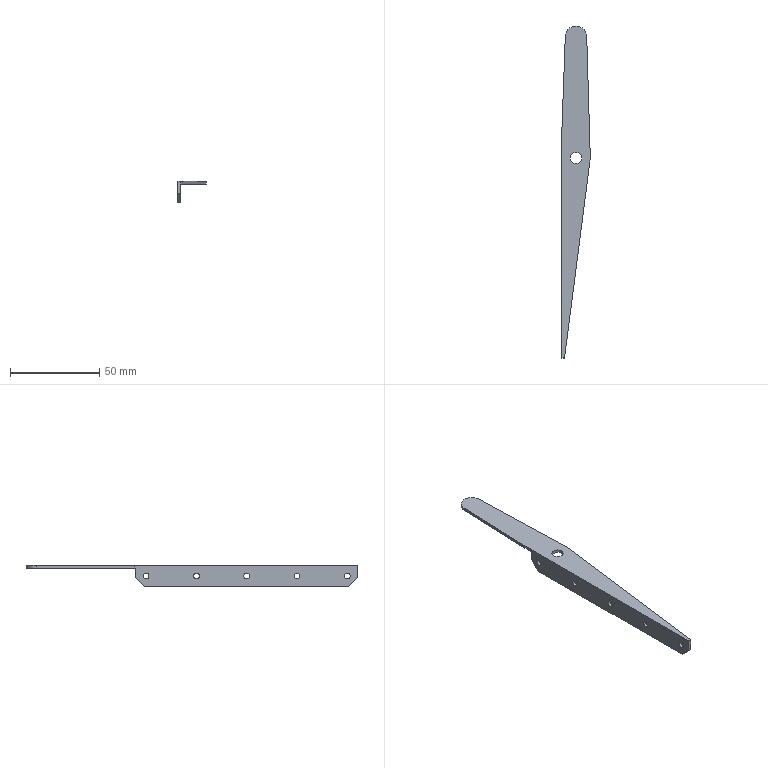Part | SolidWorks | features BaseBody 1 | 1 solid | 25 faces | box 16 x 185.958 x 12 mm | volume 5128 mm3 | cylinder 13 | plane 12 | commonest cylinder face diameters 3.2 x10 6.35 x2 12 x1
STEP:
#1=CARTESIAN_POINT('',(0.,90.45,-7.6));
#2=VERTEX_POINT('',#1);
#3=CARTESIAN_POINT('',(0.,90.45,-4.4));
#4=VERTEX_POINT('',#3);
#5=CARTESIAN_POINT('',(0.,90.45,-6.));
#6=DIRECTION('',(-1.,0.,0.));
#7=DIRECTION('',(0.,0.,-1.));
#8=AXIS2_PLACEMENT_3D('',#5,#6,#7);
#9=CIRCLE('',#8,1.6);
#10=EDGE_CURVE('',#2,#4,#9,.T.);
#11=ORIENTED_EDGE('',*,*,#10,.T.);
#12=CARTESIAN_POINT('',(1.6,90.45,-4.4));
#13=VERTEX_POINT('',#12);
#14=CARTESIAN_POINT('',(0.,90.45,-4.4));
#15=DIRECTION('',(1.,0.,0.));
#16=VECTOR('',#15,1000.);
#17=LINE('',#14,#16);
#18=EDGE_CURVE('',#4,#13,#17,.T.);
#19=ORIENTED_EDGE('',*,*,#18,.T.);
#20=CARTESIAN_POINT('',(1.6,90.45,-7.6));
#21=VERTEX_POINT('',#20);
#22=CARTESIAN_POINT('',(1.6,90.45,-6.));
#23=DIRECTION('',(1.,0.,0.));
#24=DIRECTION('',(0.,0.,-1.));
#25=AXIS2_PLACEMENT_3D('',#22,#23,#24);
#26=CIRCLE('',#25,1.6);
#27=EDGE_CURVE('',#13,#21,#26,.T.);
#28=ORIENTED_EDGE('',*,*,#27,.T.);
#29=CARTESIAN_POINT('',(0.,90.45,-7.6));
#30=DIRECTION('',(1.,0.,0.));
#31=VECTOR('',#30,1000.);
#32=LINE('',#29,#31);
#33=EDGE_CURVE('',#2,#21,#32,.T.);
#34=ORIENTED_EDGE('',*,*,#33,.F.);
#35=EDGE_LOOP('',(#11,#19,#28,#34));
#36=FACE_OUTER_BOUND('',#35,.T.);
#37=CARTESIAN_POINT('',(0.,90.45,-6.));
#38=DIRECTION('',(1.,0.,0.));
#39=DIRECTION('',(0.,0.,-1.));
#40=AXIS2_PLACEMENT_3D('',#37,#38,#39);
#41=CYLINDRICAL_SURFACE('',#40,1.6);
#42=ADVANCED_FACE('',(#36),#41,.F.);
#43=CARTESIAN_POINT('',(0.,118.645,-7.6));
#44=VERTEX_POINT('',#43);
#45=CARTESIAN_POINT('',(0.,118.645,-4.4));
#46=VERTEX_POINT('',#45);
#47=CARTESIAN_POINT('',(0.,118.645,-6.));
#48=DIRECTION('',(-1.,0.,0.));
#49=DIRECTION('',(0.,0.,-1.));
#50=AXIS2_PLACEMENT_3D('',#47,#48,#49);
#51=CIRCLE('',#50,1.6);
#52=EDGE_CURVE('',#44,#46,#51,.T.);
#53=ORIENTED_EDGE('',*,*,#52,.T.);
#54=CARTESIAN_POINT('',(1.6,118.645,-4.4));
#55=VERTEX_POINT('',#54);
#56=CARTESIAN_POINT('',(0.,118.645,-4.4));
#57=DIRECTION('',(1.,0.,0.));
#58=VECTOR('',#57,1000.);
#59=LINE('',#56,#58);
#60=EDGE_CURVE('',#46,#55,#59,.T.);
#61=ORIENTED_EDGE('',*,*,#60,.T.);
#62=CARTESIAN_POINT('',(1.6,118.645,-7.6));
#63=VERTEX_POINT('',#62);
#64=CARTESIAN_POINT('',(1.6,118.645,-6.));
#65=DIRECTION('',(1.,0.,0.));
#66=DIRECTION('',(0.,0.,-1.));
#67=AXIS2_PLACEMENT_3D('',#64,#65,#66);
#68=CIRCLE('',#67,1.6);
#69=EDGE_CURVE('',#55,#63,#68,.T.);
#70=ORIENTED_EDGE('',*,*,#69,.T.);
#71=CARTESIAN_POINT('',(0.,118.645,-7.6));
#72=DIRECTION('',(1.,0.,0.));
#73=VECTOR('',#72,1000.);
#74=LINE('',#71,#73);
#75=EDGE_CURVE('',#44,#63,#74,.T.);
#76=ORIENTED_EDGE('',*,*,#75,.F.);
#77=EDGE_LOOP('',(#53,#61,#70,#76));
#78=FACE_OUTER_BOUND('',#77,.T.);
#79=CARTESIAN_POINT('',(0.,118.645,-6.));
#80=DIRECTION('',(1.,0.,0.));
#81=DIRECTION('',(0.,0.,-1.));
#82=AXIS2_PLACEMENT_3D('',#79,#80,#81);
#83=CYLINDRICAL_SURFACE('',#82,1.6);
#84=ADVANCED_FACE('',(#78),#83,.F.);
#85=CARTESIAN_POINT('',(0.,34.15,-7.6));
#86=VERTEX_POINT('',#85);
#87=CARTESIAN_POINT('',(0.,34.15,-4.4));
#88=VERTEX_POINT('',#87);
#89=CARTESIAN_POINT('',(0.,34.15,-6.));
#90=DIRECTION('',(-1.,0.,0.));
#91=DIRECTION('',(0.,0.,-1.));
#92=AXIS2_PLACEMENT_3D('',#89,#90,#91);
#93=CIRCLE('',#92,1.6);
#94=EDGE_CURVE('',#86,#88,#93,.T.);
#95=ORIENTED_EDGE('',*,*,#94,.T.);
#96=CARTESIAN_POINT('',(1.6,34.15,-4.4));
#97=VERTEX_POINT('',#96);
#98=CARTESIAN_POINT('',(0.,34.15,-4.4));
#99=DIRECTION('',(1.,0.,0.));
#100=VECTOR('',#99,1000.);
#101=LINE('',#98,#100);
#102=EDGE_CURVE('',#88,#97,#101,.T.);
#103=ORIENTED_EDGE('',*,*,#102,.T.);
#104=CARTESIAN_POINT('',(1.6,34.15,-7.6));
#105=VERTEX_POINT('',#104);
#106=CARTESIAN_POINT('',(1.6,34.15,-6.));
#107=DIRECTION('',(1.,0.,0.));
#108=DIRECTION('',(0.,0.,-1.));
#109=AXIS2_PLACEMENT_3D('',#106,#107,#108);
#110=CIRCLE('',#109,1.6);
#111=EDGE_CURVE('',#97,#105,#110,.T.);
#112=ORIENTED_EDGE('',*,*,#111,.T.);
#113=CARTESIAN_POINT('',(0.,34.15,-7.6));
#114=DIRECTION('',(1.,0.,0.));
#115=VECTOR('',#114,1000.);
#116=LINE('',#113,#115);
#117=EDGE_CURVE('',#86,#105,#116,.T.);
#118=ORIENTED_EDGE('',*,*,#117,.F.);
#119=EDGE_LOOP('',(#95,#103,#112,#118));
#120=FACE_OUTER_BOUND('',#119,.T.);
#121=CARTESIAN_POINT('',(0.,34.15,-6.));
#122=DIRECTION('',(1.,0.,0.));
#123=DIRECTION('',(0.,0.,-1.));
#124=AXIS2_PLACEMENT_3D('',#121,#122,#123);
#125=CYLINDRICAL_SURFACE('',#124,1.6);
#126=ADVANCED_FACE('',(#120),#125,.F.);
#127=CARTESIAN_POINT('',(0.,6.,-7.6));
#128=VERTEX_POINT('',#127);
#129=CARTESIAN_POINT('',(0.,6.,-4.4));
#130=VERTEX_POINT('',#129);
#131=CARTESIAN_POINT('',(0.,6.,-6.));
#132=DIRECTION('',(-1.,0.,0.));
#133=DIRECTION('',(0.,0.,-1.));
#134=AXIS2_PLACEMENT_3D('',#131,#132,#133);
#135=CIRCLE('',#134,1.6);
#136=EDGE_CURVE('',#128,#130,#135,.T.);
#137=ORIENTED_EDGE('',*,*,#136,.T.);
#138=CARTESIAN_POINT('',(1.6,6.,-4.4));
#139=VERTEX_POINT('',#138);
#140=CARTESIAN_POINT('',(0.,6.,-4.4));
#141=DIRECTION('',(1.,0.,0.));
#142=VECTOR('',#141,1000.);
#143=LINE('',#140,#142);
#144=EDGE_CURVE('',#130,#139,#143,.T.);
#145=ORIENTED_EDGE('',*,*,#144,.T.);
#146=CARTESIAN_POINT('',(1.6,6.,-7.6));
#147=VERTEX_POINT('',#146);
#148=CARTESIAN_POINT('',(1.6,6.,-6.));
#149=DIRECTION('',(1.,0.,0.));
#150=DIRECTION('',(0.,0.,-1.));
#151=AXIS2_PLACEMENT_3D('',#148,#149,#150);
#152=CIRCLE('',#151,1.6);
#153=EDGE_CURVE('',#139,#147,#152,.T.);
#154=ORIENTED_EDGE('',*,*,#153,.T.);
#155=CARTESIAN_POINT('',(0.,6.,-7.6));
#156=DIRECTION('',(1.,0.,0.));
#157=VECTOR('',#156,1000.);
#158=LINE('',#155,#157);
#159=EDGE_CURVE('',#128,#147,#158,.T.);
#160=ORIENTED_EDGE('',*,*,#159,.F.);
#161=EDGE_LOOP('',(#137,#145,#154,#160));
#162=FACE_OUTER_BOUND('',#161,.T.);
#163=CARTESIAN_POINT('',(0.,6.,-6.));
#164=DIRECTION('',(1.,0.,0.));
#165=DIRECTION('',(0.,0.,-1.));
#166=AXIS2_PLACEMENT_3D('',#163,#164,#165);
#167=CYLINDRICAL_SURFACE('',#166,1.6);
#168=ADVANCED_FACE('',(#162),#167,.F.);
#169=CARTESIAN_POINT('',(0.,62.3,-7.6));
#170=VERTEX_POINT('',#169);
#171=CARTESIAN_POINT('',(0.,62.3,-4.4));
#172=VERTEX_POINT('',#171);
#173=CARTESIAN_POINT('',(0.,62.3,-6.));
#174=DIRECTION('',(-1.,0.,0.));
#175=DIRECTION('',(0.,0.,-1.));
#176=AXIS2_PLACEMENT_3D('',#173,#174,#175);
#177=CIRCLE('',#176,1.6);
#178=EDGE_CURVE('',#170,#172,#177,.T.);
#179=ORIENTED_EDGE('',*,*,#178,.T.);
#180=CARTESIAN_POINT('',(1.6,62.3,-4.4));
#181=VERTEX_POINT('',#180);
#182=CARTESIAN_POINT('',(0.,62.3,-4.4));
#183=DIRECTION('',(1.,0.,0.));
#184=VECTOR('',#183,1000.);
#185=LINE('',#182,#184);
#186=EDGE_CURVE('',#172,#181,#185,.T.);
#187=ORIENTED_EDGE('',*,*,#186,.T.);
#188=CARTESIAN_POINT('',(1.6,62.3,-7.6));
#189=VERTEX_POINT('',#188);
#190=CARTESIAN_POINT('',(1.6,62.3,-6.));
#191=DIRECTION('',(1.,0.,0.));
#192=DIRECTION('',(0.,0.,-1.));
#193=AXIS2_PLACEMENT_3D('',#190,#191,#192);
#194=CIRCLE('',#193,1.6);
#195=EDGE_CURVE('',#181,#189,#194,.T.);
#196=ORIENTED_EDGE('',*,*,#195,.T.);
#197=CARTESIAN_POINT('',(0.,62.3,-7.6));
#198=DIRECTION('',(1.,0.,0.));
#199=VECTOR('',#198,1000.);
#200=LINE('',#197,#199);
#201=EDGE_CURVE('',#170,#189,#200,.T.);
#202=ORIENTED_EDGE('',*,*,#201,.F.);
#203=EDGE_LOOP('',(#179,#187,#196,#202));
#204=FACE_OUTER_BOUND('',#203,.T.);
#205=CARTESIAN_POINT('',(0.,62.3,-6.));
#206=DIRECTION('',(1.,0.,0.));
#207=DIRECTION('',(0.,0.,-1.));
#208=AXIS2_PLACEMENT_3D('',#205,#206,#207);
#209=CYLINDRICAL_SURFACE('',#208,1.6);
#210=ADVANCED_FACE('',(#204),#209,.F.);
#211=CARTESIAN_POINT('',(4.825,112.,0.));
#212=VERTEX_POINT('',#211);
#213=CARTESIAN_POINT('',(11.175,112.,0.));
#214=VERTEX_POINT('',#213);
#215=CARTESIAN_POINT('',(8.,112.,0.));
#216=DIRECTION('',(0.,0.,1.));
#217=DIRECTION('',(-1.,0.,0.));
#218=AXIS2_PLACEMENT_3D('',#215,#216,#217);
#219=CIRCLE('',#218,3.175);
#220=EDGE_CURVE('',#212,#214,#219,.T.);
#221=ORIENTED_EDGE('',*,*,#220,.T.);
#222=CARTESIAN_POINT('',(11.175,112.,-1.6));
#223=VERTEX_POINT('',#222);
#224=CARTESIAN_POINT('',(11.175,112.,0.));
#225=DIRECTION('',(0.,0.,-1.));
#226=VECTOR('',#225,1000.);
#227=LINE('',#224,#226);
#228=EDGE_CURVE('',#214,#223,#227,.T.);
#229=ORIENTED_EDGE('',*,*,#228,.T.);
#230=CARTESIAN_POINT('',(4.825,112.,-1.6));
#231=VERTEX_POINT('',#230);
#232=CARTESIAN_POINT('',(8.,112.,-1.6));
#233=DIRECTION('',(0.,0.,-1.));
#234=DIRECTION('',(-1.,0.,0.));
#235=AXIS2_PLACEMENT_3D('',#232,#233,#234);
#236=CIRCLE('',#235,3.175);
#237=EDGE_CURVE('',#223,#231,#236,.T.);
#238=ORIENTED_EDGE('',*,*,#237,.T.);
#239=CARTESIAN_POINT('',(4.825,112.,0.));
#240=DIRECTION('',(0.,0.,-1.));
#241=VECTOR('',#240,1000.);
#242=LINE('',#239,#241);
#243=EDGE_CURVE('',#212,#231,#242,.T.);
#244=ORIENTED_EDGE('',*,*,#243,.F.);
#245=EDGE_LOOP('',(#221,#229,#238,#244));
#246=FACE_OUTER_BOUND('',#245,.T.);
#247=CARTESIAN_POINT('',(8.,112.,0.));
#248=DIRECTION('',(0.,0.,-1.));
#249=DIRECTION('',(-1.,0.,0.));
#250=AXIS2_PLACEMENT_3D('',#247,#248,#249);
#251=CYLINDRICAL_SURFACE('',#250,3.175);
#252=ADVANCED_FACE('',(#246),#251,.F.);
#253=ORIENTED_EDGE('',*,*,#18,.F.);
#254=CARTESIAN_POINT('',(0.,90.45,-6.));
#255=DIRECTION('',(-1.,0.,0.));
#256=DIRECTION('',(0.,0.,-1.));
#257=AXIS2_PLACEMENT_3D('',#254,#255,#256);
#258=CIRCLE('',#257,1.6);
#259=EDGE_CURVE('',#4,#2,#258,.T.);
#260=ORIENTED_EDGE('',*,*,#259,.T.);
#261=ORIENTED_EDGE('',*,*,#33,.T.);
#262=CARTESIAN_POINT('',(1.6,90.45,-6.));
#263=DIRECTION('',(1.,0.,0.));
#264=DIRECTION('',(0.,0.,-1.));
#265=AXIS2_PLACEMENT_3D('',#262,#263,#264);
#266=CIRCLE('',#265,1.6);
#267=EDGE_CURVE('',#21,#13,#266,.T.);
#268=ORIENTED_EDGE('',*,*,#267,.T.);
#269=EDGE_LOOP('',(#253,#260,#261,#268));
#270=FACE_OUTER_BOUND('',#269,.T.);
#271=CARTESIAN_POINT('',(0.,90.45,-6.));
#272=DIRECTION('',(1.,0.,0.));
#273=DIRECTION('',(0.,0.,-1.));
#274=AXIS2_PLACEMENT_3D('',#271,#272,#273);
#275=CYLINDRICAL_SURFACE('',#274,1.6);
#276=ADVANCED_FACE('',(#270),#275,.F.);
#277=CARTESIAN_POINT('',(1.6,118.645,-6.));
#278=DIRECTION('',(1.,0.,0.));
#279=DIRECTION('',(0.,0.,-1.));
#280=AXIS2_PLACEMENT_3D('',#277,#278,#279);
#281=CIRCLE('',#280,1.6);
#282=EDGE_CURVE('',#63,#55,#281,.T.);
#283=ORIENTED_EDGE('',*,*,#282,.F.);
#284=ORIENTED_EDGE('',*,*,#69,.F.);
#285=EDGE_LOOP('',(#283,#284));
#286=FACE_BOUND('',#285,.T.);
#287=CARTESIAN_POINT('',(1.6,34.15,-6.));
#288=DIRECTION('',(1.,0.,0.));
#289=DIRECTION('',(0.,0.,-1.));
#290=AXIS2_PLACEMENT_3D('',#287,#288,#289);
#291=CIRCLE('',#290,1.6);
#292=EDGE_CURVE('',#105,#97,#291,.T.);
#293=ORIENTED_EDGE('',*,*,#292,.F.);
#294=ORIENTED_EDGE('',*,*,#111,.F.);
#295=EDGE_LOOP('',(#293,#294));
#296=FACE_BOUND('',#295,.T.);
#297=CARTESIAN_POINT('',(1.6,6.,-6.));
#298=DIRECTION('',(1.,0.,0.));
#299=DIRECTION('',(0.,0.,-1.));
#300=AXIS2_PLACEMENT_3D('',#297,#298,#299);
#301=CIRCLE('',#300,1.6);
#302=EDGE_CURVE('',#147,#139,#301,.T.);
#303=ORIENTED_EDGE('',*,*,#302,.F.);
#304=ORIENTED_EDGE('',*,*,#153,.F.);
#305=EDGE_LOOP('',(#303,#304));
#306=FACE_BOUND('',#305,.T.);
#307=CARTESIAN_POINT('',(1.6,62.3,-6.));
#308=DIRECTION('',(1.,0.,0.));
#309=DIRECTION('',(0.,0.,-1.));
#310=AXIS2_PLACEMENT_3D('',#307,#308,#309);
#311=CIRCLE('',#310,1.6);
#312=EDGE_CURVE('',#189,#181,#311,.T.);
#313=ORIENTED_EDGE('',*,*,#312,.F.);
#314=ORIENTED_EDGE('',*,*,#195,.F.);
#315=EDGE_LOOP('',(#313,#314));
#316=FACE_BOUND('',#315,.T.);
#317=ORIENTED_EDGE('',*,*,#267,.F.);
#318=ORIENTED_EDGE('',*,*,#27,.F.);
#319=EDGE_LOOP('',(#317,#318));
#320=FACE_BOUND('',#319,.T.);
#321=CARTESIAN_POINT('',(1.6,0.,-6.8));
#322=VERTEX_POINT('',#321);
#323=CARTESIAN_POINT('',(1.6,0.,-1.6));
#324=VERTEX_POINT('',#323);
#325=CARTESIAN_POINT('',(1.6,0.,-6.8));
#326=DIRECTION('',(0.,0.,1.));
#327=VECTOR('',#326,1000.);
#328=LINE('',#325,#327);
#329=EDGE_CURVE('',#322,#324,#328,.T.);
#330=ORIENTED_EDGE('',*,*,#329,.F.);
#331=CARTESIAN_POINT('',(1.6,5.2,-12.));
#332=VERTEX_POINT('',#331);
#333=CARTESIAN_POINT('',(1.6,0.,-6.8));
#334=DIRECTION('',(0.,-0.7071,0.7071));
#335=VECTOR('',#334,1000.);
#336=LINE('',#333,#335);
#337=EDGE_CURVE('',#332,#322,#336,.T.);
#338=ORIENTED_EDGE('',*,*,#337,.F.);
#339=CARTESIAN_POINT('',(1.6,119.8,-12.));
#340=VERTEX_POINT('',#339);
#341=CARTESIAN_POINT('',(1.6,62.323,-12.));
#342=DIRECTION('',(0.,-1.,0.));
#343=VECTOR('',#342,1000.);
#344=LINE('',#341,#343);
#345=EDGE_CURVE('',#340,#332,#344,.T.);
#346=ORIENTED_EDGE('',*,*,#345,.F.);
#347=CARTESIAN_POINT('',(1.6,124.645,-6.801));
#348=VERTEX_POINT('',#347);
#349=CARTESIAN_POINT('',(1.6,119.8,-12.));
#350=DIRECTION('',(0.,-0.6818,-0.7316));
#351=VECTOR('',#350,1000.);
#352=LINE('',#349,#351);
#353=EDGE_CURVE('',#348,#340,#352,.T.);
#354=ORIENTED_EDGE('',*,*,#353,.F.);
#355=CARTESIAN_POINT('',(1.6,124.645,-1.6));
#356=VERTEX_POINT('',#355);
#357=CARTESIAN_POINT('',(1.6,124.645,-6.8));
#358=DIRECTION('',(0.,0.,-1.));
#359=VECTOR('',#358,1000.);
#360=LINE('',#357,#359);
#361=EDGE_CURVE('',#356,#348,#360,.T.);
#362=ORIENTED_EDGE('',*,*,#361,.F.);
#363=CARTESIAN_POINT('',(1.6,62.323,-1.6));
#364=DIRECTION('',(0.,1.,0.));
#365=VECTOR('',#364,1000.);
#366=LINE('',#363,#365);
#367=EDGE_CURVE('',#324,#356,#366,.T.);
#368=ORIENTED_EDGE('',*,*,#367,.F.);
#369=EDGE_LOOP('',(#330,#338,#346,#354,#362,#368));
#370=FACE_OUTER_BOUND('',#369,.T.);
#371=CARTESIAN_POINT('',(1.6,124.645,-1.6));
#372=DIRECTION('',(-1.,0.,0.));
#373=DIRECTION('',(0.,0.,-1.));
#374=AXIS2_PLACEMENT_3D('',#371,#372,#373);
#375=PLANE('',#374);
#376=ADVANCED_FACE('',(#286,#296,#306,#316,#320,#370),#375,.F.);
#377=ORIENTED_EDGE('',*,*,#52,.F.);
#378=CARTESIAN_POINT('',(0.,118.645,-6.));
#379=DIRECTION('',(-1.,0.,0.));
#380=DIRECTION('',(0.,0.,-1.));
#381=AXIS2_PLACEMENT_3D('',#378,#379,#380);
#382=CIRCLE('',#381,1.6);
#383=EDGE_CURVE('',#46,#44,#382,.T.);
#384=ORIENTED_EDGE('',*,*,#383,.F.);
#385=EDGE_LOOP('',(#377,#384));
#386=FACE_BOUND('',#385,.T.);
#387=ORIENTED_EDGE('',*,*,#94,.F.);
#388=CARTESIAN_POINT('',(0.,34.15,-6.));
#389=DIRECTION('',(-1.,0.,0.));
#390=DIRECTION('',(0.,0.,-1.));
#391=AXIS2_PLACEMENT_3D('',#388,#389,#390);
#392=CIRCLE('',#391,1.6);
#393=EDGE_CURVE('',#88,#86,#392,.T.);
#394=ORIENTED_EDGE('',*,*,#393,.F.);
#395=EDGE_LOOP('',(#387,#394));
#396=FACE_BOUND('',#395,.T.);
#397=ORIENTED_EDGE('',*,*,#136,.F.);
#398=CARTESIAN_POINT('',(0.,6.,-6.));
#399=DIRECTION('',(-1.,0.,0.));
#400=DIRECTION('',(0.,0.,-1.));
#401=AXIS2_PLACEMENT_3D('',#398,#399,#400);
#402=CIRCLE('',#401,1.6);
#403=EDGE_CURVE('',#130,#128,#402,.T.);
#404=ORIENTED_EDGE('',*,*,#403,.F.);
#405=EDGE_LOOP('',(#397,#404));
#406=FACE_BOUND('',#405,.T.);
#407=ORIENTED_EDGE('',*,*,#178,.F.);
#408=CARTESIAN_POINT('',(0.,62.3,-6.));
#409=DIRECTION('',(-1.,0.,0.));
#410=DIRECTION('',(0.,0.,-1.));
#411=AXIS2_PLACEMENT_3D('',#408,#409,#410);
#412=CIRCLE('',#411,1.6);
#413=EDGE_CURVE('',#172,#170,#412,.T.);
#414=ORIENTED_EDGE('',*,*,#413,.F.);
#415=EDGE_LOOP('',(#407,#414));
#416=FACE_BOUND('',#415,.T.);
#417=ORIENTED_EDGE('',*,*,#10,.F.);
#418=ORIENTED_EDGE('',*,*,#259,.F.);
#419=EDGE_LOOP('',(#417,#418));
#420=FACE_BOUND('',#419,.T.);
#421=CARTESIAN_POINT('',(0.,119.8,-12.));
#422=VERTEX_POINT('',#421);
#423=CARTESIAN_POINT('',(0.,124.645,-6.801));
#424=VERTEX_POINT('',#423);
#425=CARTESIAN_POINT('',(0.,119.8,-12.));
#426=DIRECTION('',(0.,0.6818,0.7316));
#427=VECTOR('',#426,1000.);
#428=LINE('',#425,#427);
#429=EDGE_CURVE('',#422,#424,#428,.T.);
#430=ORIENTED_EDGE('',*,*,#429,.F.);
#431=CARTESIAN_POINT('',(0.,5.2,-12.));
#432=VERTEX_POINT('',#431);
#433=CARTESIAN_POINT('',(0.,62.5,-12.));
#434=DIRECTION('',(0.,1.,0.));
#435=VECTOR('',#434,1000.);
#436=LINE('',#433,#435);
#437=EDGE_CURVE('',#432,#422,#436,.T.);
#438=ORIENTED_EDGE('',*,*,#437,.F.);
#439=CARTESIAN_POINT('',(0.,0.,-6.8));
#440=VERTEX_POINT('',#439);
#441=CARTESIAN_POINT('',(0.,0.,-6.8));
#442=DIRECTION('',(0.,0.7071,-0.7071));
#443=VECTOR('',#442,1000.);
#444=LINE('',#441,#443);
#445=EDGE_CURVE('',#440,#432,#444,.T.);
#446=ORIENTED_EDGE('',*,*,#445,.F.);
#447=CARTESIAN_POINT('',(0.,0.,0.));
#448=VERTEX_POINT('',#447);
#449=CARTESIAN_POINT('',(0.,0.,-6.));
#450=DIRECTION('',(0.,0.,-1.));
#451=VECTOR('',#450,1000.);
#452=LINE('',#449,#451);
#453=EDGE_CURVE('',#448,#440,#452,.T.);
#454=ORIENTED_EDGE('',*,*,#453,.F.);
#455=CARTESIAN_POINT('',(0.,125.,0.));
#456=VERTEX_POINT('',#455);
#457=CARTESIAN_POINT('',(0.,62.5,0.));
#458=DIRECTION('',(0.,-1.,0.));
#459=VECTOR('',#458,1000.);
#460=LINE('',#457,#459);
#461=EDGE_CURVE('',#456,#448,#460,.T.);
#462=ORIENTED_EDGE('',*,*,#461,.F.);
#463=CARTESIAN_POINT('',(0.,125.,-1.6));
#464=VERTEX_POINT('',#463);
#465=CARTESIAN_POINT('',(0.,125.,-0.8));
#466=DIRECTION('',(0.,0.,-1.));
#467=VECTOR('',#466,1000.);
#468=LINE('',#465,#467);
#469=EDGE_CURVE('',#456,#464,#468,.T.);
#470=ORIENTED_EDGE('',*,*,#469,.T.);
#471=CARTESIAN_POINT('',(0.,124.645,-1.6));
#472=VERTEX_POINT('',#471);
#473=CARTESIAN_POINT('',(0.,62.5,-1.6));
#474=DIRECTION('',(0.,1.,0.));
#475=VECTOR('',#474,1000.);
#476=LINE('',#473,#475);
#477=EDGE_CURVE('',#472,#464,#476,.T.);
#478=ORIENTED_EDGE('',*,*,#477,.F.);
#479=CARTESIAN_POINT('',(0.,124.645,-6.));
#480=DIRECTION('',(0.,0.,1.));
#481=VECTOR('',#480,1000.);
#482=LINE('',#479,#481);
#483=EDGE_CURVE('',#424,#472,#482,.T.);
#484=ORIENTED_EDGE('',*,*,#483,.F.);
#485=EDGE_LOOP('',(#430,#438,#446,#454,#462,#470,#478,#484));
#486=FACE_OUTER_BOUND('',#485,.T.);
#487=CARTESIAN_POINT('',(0.,125.,-12.));
#488=DIRECTION('',(1.,0.,0.));
#489=DIRECTION('',(0.,0.,1.));
#490=AXIS2_PLACEMENT_3D('',#487,#488,#489);
#491=PLANE('',#490);
#492=ADVANCED_FACE('',(#386,#396,#406,#416,#420,#486),#491,.F.);
#493=ORIENTED_EDGE('',*,*,#60,.F.);
#494=ORIENTED_EDGE('',*,*,#383,.T.);
#495=ORIENTED_EDGE('',*,*,#75,.T.);
#496=ORIENTED_EDGE('',*,*,#282,.T.);
#497=EDGE_LOOP('',(#493,#494,#495,#496));
#498=FACE_OUTER_BOUND('',#497,.T.);
#499=CARTESIAN_POINT('',(0.,118.645,-6.));
#500=DIRECTION('',(1.,0.,0.));
#501=DIRECTION('',(0.,0.,-1.));
#502=AXIS2_PLACEMENT_3D('',#499,#500,#501);
#503=CYLINDRICAL_SURFACE('',#502,1.6);
#504=ADVANCED_FACE('',(#498),#503,.F.);
#505=ORIENTED_EDGE('',*,*,#102,.F.);
#506=ORIENTED_EDGE('',*,*,#393,.T.);
#507=ORIENTED_EDGE('',*,*,#117,.T.);
#508=ORIENTED_EDGE('',*,*,#292,.T.);
#509=EDGE_LOOP('',(#505,#506,#507,#508));
#510=FACE_OUTER_BOUND('',#509,.T.);
#511=CARTESIAN_POINT('',(0.,34.15,-6.));
#512=DIRECTION('',(1.,0.,0.));
#513=DIRECTION('',(0.,0.,-1.));
#514=AXIS2_PLACEMENT_3D('',#511,#512,#513);
#515=CYLINDRICAL_SURFACE('',#514,1.6);
#516=ADVANCED_FACE('',(#510),#515,.F.);
#517=ORIENTED_EDGE('',*,*,#144,.F.);
#518=ORIENTED_EDGE('',*,*,#403,.T.);
#519=ORIENTED_EDGE('',*,*,#159,.T.);
#520=ORIENTED_EDGE('',*,*,#302,.T.);
#521=EDGE_LOOP('',(#517,#518,#519,#520));
#522=FACE_OUTER_BOUND('',#521,.T.);
#523=CARTESIAN_POINT('',(0.,6.,-6.));
#524=DIRECTION('',(1.,0.,0.));
#525=DIRECTION('',(0.,0.,-1.));
#526=AXIS2_PLACEMENT_3D('',#523,#524,#525);
#527=CYLINDRICAL_SURFACE('',#526,1.6);
#528=ADVANCED_FACE('',(#522),#527,.F.);
#529=ORIENTED_EDGE('',*,*,#186,.F.);
#530=ORIENTED_EDGE('',*,*,#413,.T.);
#531=ORIENTED_EDGE('',*,*,#201,.T.);
#532=ORIENTED_EDGE('',*,*,#312,.T.);
#533=EDGE_LOOP('',(#529,#530,#531,#532));
#534=FACE_OUTER_BOUND('',#533,.T.);
#535=CARTESIAN_POINT('',(0.,62.3,-6.));
#536=DIRECTION('',(1.,0.,0.));
#537=DIRECTION('',(0.,0.,-1.));
#538=AXIS2_PLACEMENT_3D('',#535,#536,#537);
#539=CYLINDRICAL_SURFACE('',#538,1.6);
#540=ADVANCED_FACE('',(#534),#539,.F.);
#541=CARTESIAN_POINT('',(8.,112.,-1.6));
#542=DIRECTION('',(0.,0.,-1.));
#543=DIRECTION('',(-1.,0.,0.));
#544=AXIS2_PLACEMENT_3D('',#541,#542,#543);
#545=CIRCLE('',#544,3.175);
#546=EDGE_CURVE('',#231,#223,#545,.T.);
#547=ORIENTED_EDGE('',*,*,#546,.F.);
#548=ORIENTED_EDGE('',*,*,#237,.F.);
#549=EDGE_LOOP('',(#547,#548));
#550=FACE_BOUND('',#549,.T.);
#551=CARTESIAN_POINT('',(14.,179.958,-1.6));
#552=VERTEX_POINT('',#551);
#553=CARTESIAN_POINT('',(2.,179.958,-1.6));
#554=VERTEX_POINT('',#553);
#555=CARTESIAN_POINT('',(8.,179.958,-1.6));
#556=DIRECTION('',(0.,0.,1.));
#557=DIRECTION('',(-1.,0.,0.));
#558=AXIS2_PLACEMENT_3D('',#555,#556,#557);
#559=CIRCLE('',#558,6.);
#560=EDGE_CURVE('',#552,#554,#559,.T.);
#561=ORIENTED_EDGE('',*,*,#560,.F.);
#562=CARTESIAN_POINT('',(16.,112.,-1.6));
#563=VERTEX_POINT('',#562);
#564=CARTESIAN_POINT('',(14.,179.958,-1.6));
#565=DIRECTION('',(-0.02942,0.9996,0.));
#566=VECTOR('',#565,1000.);
#567=LINE('',#564,#566);
#568=EDGE_CURVE('',#563,#552,#567,.T.);
#569=ORIENTED_EDGE('',*,*,#568,.F.);
#570=CARTESIAN_POINT('',(16.,112.,-1.6));
#571=DIRECTION('',(0.1275,0.9918,0.));
#572=VECTOR('',#571,1000.);
#573=LINE('',#570,#572);
#574=EDGE_CURVE('',#324,#563,#573,.T.);
#575=ORIENTED_EDGE('',*,*,#574,.F.);
#576=ORIENTED_EDGE('',*,*,#367,.T.);
#577=CARTESIAN_POINT('',(8.048,124.645,-1.6));
#578=DIRECTION('',(1.,0.,0.));
#579=VECTOR('',#578,1000.);
#580=LINE('',#577,#579);
#581=EDGE_CURVE('',#472,#356,#580,.T.);
#582=ORIENTED_EDGE('',*,*,#581,.F.);
#583=ORIENTED_EDGE('',*,*,#477,.T.);
#584=CARTESIAN_POINT('',(0.,125.,-1.6));
#585=DIRECTION('',(-0.03637,-0.9993,0.));
#586=VECTOR('',#585,1000.);
#587=LINE('',#584,#586);
#588=EDGE_CURVE('',#554,#464,#587,.T.);
#589=ORIENTED_EDGE('',*,*,#588,.F.);
#590=EDGE_LOOP('',(#561,#569,#575,#576,#582,#583,#589));
#591=FACE_OUTER_BOUND('',#590,.T.);
#592=CARTESIAN_POINT('',(16.096,187.073,-1.6));
#593=DIRECTION('',(0.,0.,1.));
#594=DIRECTION('',(-1.,0.,0.));
#595=AXIS2_PLACEMENT_3D('',#592,#593,#594);
#596=PLANE('',#595);
#597=ADVANCED_FACE('',(#550,#591),#596,.F.);
#598=CARTESIAN_POINT('',(1.6,0.,0.));
#599=VERTEX_POINT('',#598);
#600=CARTESIAN_POINT('',(1.6,0.,-3.4));
#601=DIRECTION('',(0.,0.,-1.));
#602=VECTOR('',#601,1000.);
#603=LINE('',#600,#602);
#604=EDGE_CURVE('',#599,#324,#603,.T.);
#605=ORIENTED_EDGE('',*,*,#604,.F.);
#606=CARTESIAN_POINT('',(0.8,0.,0.));
#607=DIRECTION('',(1.,0.,0.));
#608=VECTOR('',#607,1000.);
#609=LINE('',#606,#608);
#610=EDGE_CURVE('',#448,#599,#609,.T.);
#611=ORIENTED_EDGE('',*,*,#610,.F.);
#612=ORIENTED_EDGE('',*,*,#453,.T.);
#613=CARTESIAN_POINT('',(0.8,0.,-6.8));
#614=DIRECTION('',(-1.,0.,0.));
#615=VECTOR('',#614,1000.);
#616=LINE('',#613,#615);
#617=EDGE_CURVE('',#322,#440,#616,.T.);
#618=ORIENTED_EDGE('',*,*,#617,.F.);
#619=ORIENTED_EDGE('',*,*,#329,.T.);
#620=EDGE_LOOP('',(#605,#611,#612,#618,#619));
#621=FACE_OUTER_BOUND('',#620,.T.);
#622=CARTESIAN_POINT('',(1.6,0.,0.));
#623=DIRECTION('',(0.,1.,0.));
#624=DIRECTION('',(0.,0.,-1.));
#625=AXIS2_PLACEMENT_3D('',#622,#623,#624);
#626=PLANE('',#625);
#627=ADVANCED_FACE('',(#621),#626,.F.);
#628=ORIENTED_EDGE('',*,*,#445,.T.);
#629=CARTESIAN_POINT('',(0.8,5.2,-12.));
#630=DIRECTION('',(-1.,0.,0.));
#631=VECTOR('',#630,1000.);
#632=LINE('',#629,#631);
#633=EDGE_CURVE('',#332,#432,#632,.T.);
#634=ORIENTED_EDGE('',*,*,#633,.F.);
#635=ORIENTED_EDGE('',*,*,#337,.T.);
#636=ORIENTED_EDGE('',*,*,#617,.T.);
#637=EDGE_LOOP('',(#628,#634,#635,#636));
#638=FACE_OUTER_BOUND('',#637,.T.);
#639=CARTESIAN_POINT('',(1.6,0.,-6.8));
#640=DIRECTION('',(0.,0.7071,0.7071));
#641=DIRECTION('',(0.,0.7071,-0.7071));
#642=AXIS2_PLACEMENT_3D('',#639,#640,#641);
#643=PLANE('',#642);
#644=ADVANCED_FACE('',(#638),#643,.F.);
#645=ORIENTED_EDGE('',*,*,#633,.T.);
#646=ORIENTED_EDGE('',*,*,#437,.T.);
#647=CARTESIAN_POINT('',(0.8,119.8,-12.));
#648=DIRECTION('',(-1.,0.,0.));
#649=VECTOR('',#648,1000.);
#650=LINE('',#647,#649);
#651=EDGE_CURVE('',#340,#422,#650,.T.);
#652=ORIENTED_EDGE('',*,*,#651,.F.);
#653=ORIENTED_EDGE('',*,*,#345,.T.);
#654=EDGE_LOOP('',(#645,#646,#652,#653));
#655=FACE_OUTER_BOUND('',#654,.T.);
#656=CARTESIAN_POINT('',(1.6,119.8,-12.));
#657=DIRECTION('',(0.,0.,1.));
#658=DIRECTION('',(-1.,0.,0.));
#659=AXIS2_PLACEMENT_3D('',#656,#657,#658);
#660=PLANE('',#659);
#661=ADVANCED_FACE('',(#655),#660,.F.);
#662=ORIENTED_EDGE('',*,*,#429,.T.);
#663=CARTESIAN_POINT('',(0.8,124.645,-6.801));
#664=DIRECTION('',(-1.,0.,0.));
#665=VECTOR('',#664,1000.);
#666=LINE('',#663,#665);
#667=EDGE_CURVE('',#348,#424,#666,.T.);
#668=ORIENTED_EDGE('',*,*,#667,.F.);
#669=ORIENTED_EDGE('',*,*,#353,.T.);
#670=ORIENTED_EDGE('',*,*,#651,.T.);
#671=EDGE_LOOP('',(#662,#668,#669,#670));
#672=FACE_OUTER_BOUND('',#671,.T.);
#673=CARTESIAN_POINT('',(1.6,119.8,-12.));
#674=DIRECTION('',(0.,-0.7316,0.6818));
#675=DIRECTION('',(0.,0.6818,0.7316));
#676=AXIS2_PLACEMENT_3D('',#673,#674,#675);
#677=PLANE('',#676);
#678=ADVANCED_FACE('',(#672),#677,.F.);
#679=ORIENTED_EDGE('',*,*,#483,.T.);
#680=ORIENTED_EDGE('',*,*,#581,.T.);
#681=ORIENTED_EDGE('',*,*,#361,.T.);
#682=ORIENTED_EDGE('',*,*,#667,.T.);
#683=EDGE_LOOP('',(#679,#680,#681,#682));
#684=FACE_OUTER_BOUND('',#683,.T.);
#685=CARTESIAN_POINT('',(1.6,124.645,-6.801));
#686=DIRECTION('',(0.,-1.,0.));
#687=DIRECTION('',(0.,0.,1.));
#688=AXIS2_PLACEMENT_3D('',#685,#686,#687);
#689=PLANE('',#688);
#690=ADVANCED_FACE('',(#684),#689,.F.);
#691=ORIENTED_EDGE('',*,*,#220,.F.);
#692=CARTESIAN_POINT('',(8.,112.,0.));
#693=DIRECTION('',(0.,0.,1.));
#694=DIRECTION('',(-1.,0.,0.));
#695=AXIS2_PLACEMENT_3D('',#692,#693,#694);
#696=CIRCLE('',#695,3.175);
#697=EDGE_CURVE('',#214,#212,#696,.T.);
#698=ORIENTED_EDGE('',*,*,#697,.F.);
#699=EDGE_LOOP('',(#691,#698));
#700=FACE_BOUND('',#699,.T.);
#701=CARTESIAN_POINT('',(2.,179.958,0.));
#702=VERTEX_POINT('',#701);
#703=CARTESIAN_POINT('',(14.,179.958,0.));
#704=VERTEX_POINT('',#703);
#705=CARTESIAN_POINT('',(8.,179.958,0.));
#706=DIRECTION('',(0.,0.,-1.));
#707=DIRECTION('',(-1.,0.,0.));
#708=AXIS2_PLACEMENT_3D('',#705,#706,#707);
#709=CIRCLE('',#708,6.);
#710=EDGE_CURVE('',#702,#704,#709,.T.);
#711=ORIENTED_EDGE('',*,*,#710,.F.);
#712=CARTESIAN_POINT('',(0.,125.,0.));
#713=DIRECTION('',(0.03637,0.9993,0.));
#714=VECTOR('',#713,1000.);
#715=LINE('',#712,#714);
#716=EDGE_CURVE('',#456,#702,#715,.T.);
#717=ORIENTED_EDGE('',*,*,#716,.F.);
#718=ORIENTED_EDGE('',*,*,#461,.T.);
#719=ORIENTED_EDGE('',*,*,#610,.T.);
#720=CARTESIAN_POINT('',(16.,112.,0.));
#721=VERTEX_POINT('',#720);
#722=CARTESIAN_POINT('',(16.,112.,0.));
#723=DIRECTION('',(-0.1275,-0.9918,0.));
#724=VECTOR('',#723,1000.);
#725=LINE('',#722,#724);
#726=EDGE_CURVE('',#721,#599,#725,.T.);
#727=ORIENTED_EDGE('',*,*,#726,.F.);
#728=CARTESIAN_POINT('',(14.,179.958,0.));
#729=DIRECTION('',(0.02942,-0.9996,0.));
#730=VECTOR('',#729,1000.);
#731=LINE('',#728,#730);
#732=EDGE_CURVE('',#704,#721,#731,.T.);
#733=ORIENTED_EDGE('',*,*,#732,.F.);
#734=EDGE_LOOP('',(#711,#717,#718,#719,#727,#733));
#735=FACE_OUTER_BOUND('',#734,.T.);
#736=CARTESIAN_POINT('',(0.,187.073,0.));
#737=DIRECTION('',(0.,0.,-1.));
#738=DIRECTION('',(1.,0.,0.));
#739=AXIS2_PLACEMENT_3D('',#736,#737,#738);
#740=PLANE('',#739);
#741=ADVANCED_FACE('',(#700,#735),#740,.F.);
#742=ORIENTED_EDGE('',*,*,#228,.F.);
#743=ORIENTED_EDGE('',*,*,#697,.T.);
#744=ORIENTED_EDGE('',*,*,#243,.T.);
#745=ORIENTED_EDGE('',*,*,#546,.T.);
#746=EDGE_LOOP('',(#742,#743,#744,#745));
#747=FACE_OUTER_BOUND('',#746,.T.);
#748=CARTESIAN_POINT('',(8.,112.,0.));
#749=DIRECTION('',(0.,0.,-1.));
#750=DIRECTION('',(-1.,0.,0.));
#751=AXIS2_PLACEMENT_3D('',#748,#749,#750);
#752=CYLINDRICAL_SURFACE('',#751,3.175);
#753=ADVANCED_FACE('',(#747),#752,.F.);
#754=ORIENTED_EDGE('',*,*,#716,.T.);
#755=CARTESIAN_POINT('',(2.,179.958,-0.8));
#756=DIRECTION('',(0.,0.,1.));
#757=VECTOR('',#756,1000.);
#758=LINE('',#755,#757);
#759=EDGE_CURVE('',#554,#702,#758,.T.);
#760=ORIENTED_EDGE('',*,*,#759,.F.);
#761=ORIENTED_EDGE('',*,*,#588,.T.);
#762=ORIENTED_EDGE('',*,*,#469,.F.);
#763=EDGE_LOOP('',(#754,#760,#761,#762));
#764=FACE_OUTER_BOUND('',#763,.T.);
#765=CARTESIAN_POINT('',(0.,125.,-1.6));
#766=DIRECTION('',(0.9993,-0.03637,0.));
#767=DIRECTION('',(0.03637,0.9993,0.));
#768=AXIS2_PLACEMENT_3D('',#765,#766,#767);
#769=PLANE('',#768);
#770=ADVANCED_FACE('',(#764),#769,.F.);
#771=ORIENTED_EDGE('',*,*,#710,.T.);
#772=CARTESIAN_POINT('',(14.,179.958,-0.8));
#773=DIRECTION('',(0.,0.,1.));
#774=VECTOR('',#773,1000.);
#775=LINE('',#772,#774);
#776=EDGE_CURVE('',#552,#704,#775,.T.);
#777=ORIENTED_EDGE('',*,*,#776,.F.);
#778=ORIENTED_EDGE('',*,*,#560,.T.);
#779=ORIENTED_EDGE('',*,*,#759,.T.);
#780=EDGE_LOOP('',(#771,#777,#778,#779));
#781=FACE_OUTER_BOUND('',#780,.T.);
#782=CARTESIAN_POINT('',(8.,179.958,0.));
#783=DIRECTION('',(0.,0.,-1.));
#784=DIRECTION('',(-1.,0.,0.));
#785=AXIS2_PLACEMENT_3D('',#782,#783,#784);
#786=CYLINDRICAL_SURFACE('',#785,6.);
#787=ADVANCED_FACE('',(#781),#786,.T.);
#788=ORIENTED_EDGE('',*,*,#732,.T.);
#789=CARTESIAN_POINT('',(16.,112.,-0.8));
#790=DIRECTION('',(0.,0.,1.));
#791=VECTOR('',#790,1000.);
#792=LINE('',#789,#791);
#793=EDGE_CURVE('',#563,#721,#792,.T.);
#794=ORIENTED_EDGE('',*,*,#793,.F.);
#795=ORIENTED_EDGE('',*,*,#568,.T.);
#796=ORIENTED_EDGE('',*,*,#776,.T.);
#797=EDGE_LOOP('',(#788,#794,#795,#796));
#798=FACE_OUTER_BOUND('',#797,.T.);
#799=CARTESIAN_POINT('',(14.,179.958,-1.6));
#800=DIRECTION('',(-0.9996,-0.02942,0.));
#801=DIRECTION('',(0.02942,-0.9996,0.));
#802=AXIS2_PLACEMENT_3D('',#799,#800,#801);
#803=PLANE('',#802);
#804=ADVANCED_FACE('',(#798),#803,.F.);
#805=ORIENTED_EDGE('',*,*,#726,.T.);
#806=ORIENTED_EDGE('',*,*,#604,.T.);
#807=ORIENTED_EDGE('',*,*,#574,.T.);
#808=ORIENTED_EDGE('',*,*,#793,.T.);
#809=EDGE_LOOP('',(#805,#806,#807,#808));
#810=FACE_OUTER_BOUND('',#809,.T.);
#811=CARTESIAN_POINT('',(16.,112.,-1.6));
#812=DIRECTION('',(-0.9918,0.1275,0.));
#813=DIRECTION('',(-0.1275,-0.9918,0.));
#814=AXIS2_PLACEMENT_3D('',#811,#812,#813);
#815=PLANE('',#814);
#816=ADVANCED_FACE('',(#810),#815,.F.);
#817=CLOSED_SHELL('',(#42,#84,#126,#168,#210,#252,#276,#376,#492,#504,#516,#528,#540,#597,#627,#644,#661,#678,#690,#741,#753,#770,#787,#804,#816));
#818=MANIFOLD_SOLID_BREP('',#817);
#819=CARTESIAN_POINT('',(0.,0.,0.));
#820=DIRECTION('',(0.,0.,1.));
#821=DIRECTION('',(1.,0.,0.));
#822=AXIS2_PLACEMENT_3D('',#819,#820,#821);
#823=(LENGTH_UNIT()NAMED_UNIT(*)SI_UNIT(.MILLI.,.METRE.));
#824=UNCERTAINTY_MEASURE_WITH_UNIT(LENGTH_MEASURE(0.00001),#823,'','');
#825=(NAMED_UNIT(*)PLANE_ANGLE_UNIT()SI_UNIT($,.RADIAN.));
#826=(NAMED_UNIT(*)SI_UNIT($,.STERADIAN.)SOLID_ANGLE_UNIT());
#827=(GEOMETRIC_REPRESENTATION_CONTEXT(3)GLOBAL_UNCERTAINTY_ASSIGNED_CONTEXT((#824))GLOBAL_UNIT_ASSIGNED_CONTEXT((#823,#825,#826))REPRESENTATION_CONTEXT('',''));
#828=ADVANCED_BREP_SHAPE_REPRESENTATION('',(#818,#822),#827);